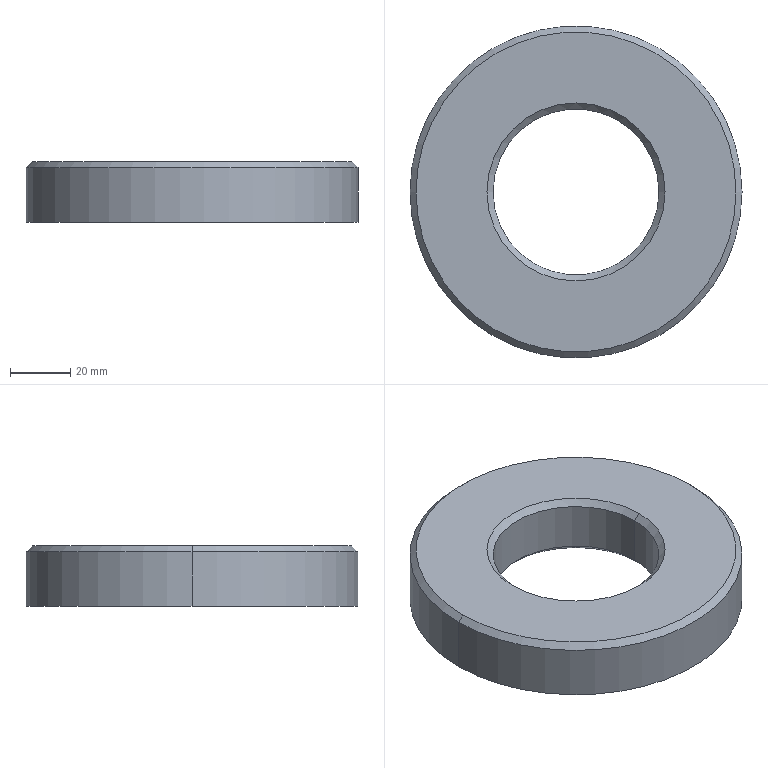Part | SolidWorks | features Chamfer 1, Extrusion 1 | 1 solid | 12 faces | box 110 x 110 x 20 mm | volume 141159 mm3 | cone 6 | cylinder 4 | plane 2 | commonest cylinder face diameters 55 x2 110 x2
STEP:
#1=CARTESIAN_POINT('',(53.,0.,20.));
#2=VERTEX_POINT('',#1);
#3=CARTESIAN_POINT('',(-53.,0.,20.));
#4=VERTEX_POINT('',#3);
#5=CARTESIAN_POINT('',(0.,0.,20.));
#6=DIRECTION('',(0.,0.,1.));
#7=DIRECTION('',(1.,0.,0.));
#8=AXIS2_PLACEMENT_3D('',#5,#6,#7);
#9=CIRCLE('',#8,53.);
#10=EDGE_CURVE('',#2,#4,#9,.T.);
#11=ORIENTED_EDGE('',*,*,#10,.F.);
#12=CARTESIAN_POINT('',(55.,0.,18.));
#13=VERTEX_POINT('',#12);
#14=CARTESIAN_POINT('',(53.,0.,20.));
#15=DIRECTION('',(0.7071,0.,-0.7071));
#16=VECTOR('',#15,1000.);
#17=LINE('',#14,#16);
#18=EDGE_CURVE('',#2,#13,#17,.T.);
#19=ORIENTED_EDGE('',*,*,#18,.T.);
#20=CARTESIAN_POINT('',(-55.,0.,18.));
#21=VERTEX_POINT('',#20);
#22=CARTESIAN_POINT('',(0.,0.,18.));
#23=DIRECTION('',(0.,0.,-1.));
#24=DIRECTION('',(1.,0.,0.));
#25=AXIS2_PLACEMENT_3D('',#22,#23,#24);
#26=CIRCLE('',#25,55.);
#27=EDGE_CURVE('',#21,#13,#26,.T.);
#28=ORIENTED_EDGE('',*,*,#27,.F.);
#29=CARTESIAN_POINT('',(-53.,0.,20.));
#30=DIRECTION('',(-0.7071,0.,-0.7071));
#31=VECTOR('',#30,1000.);
#32=LINE('',#29,#31);
#33=EDGE_CURVE('',#4,#21,#32,.T.);
#34=ORIENTED_EDGE('',*,*,#33,.F.);
#35=EDGE_LOOP('',(#11,#19,#28,#34));
#36=FACE_OUTER_BOUND('',#35,.T.);
#37=CARTESIAN_POINT('',(0.,0.,20.));
#38=DIRECTION('',(0.,0.,-1.));
#39=DIRECTION('',(-1.,0.,0.));
#40=AXIS2_PLACEMENT_3D('',#37,#38,#39);
#41=CONICAL_SURFACE('',#40,53.,0.7854);
#42=ADVANCED_FACE('',(#36),#41,.T.);
#43=CARTESIAN_POINT('',(-27.5,0.,18.));
#44=VERTEX_POINT('',#43);
#45=CARTESIAN_POINT('',(27.5,0.,18.));
#46=VERTEX_POINT('',#45);
#47=CARTESIAN_POINT('',(0.,0.,18.));
#48=DIRECTION('',(0.,0.,1.));
#49=DIRECTION('',(1.,0.,0.));
#50=AXIS2_PLACEMENT_3D('',#47,#48,#49);
#51=CIRCLE('',#50,27.5);
#52=EDGE_CURVE('',#44,#46,#51,.T.);
#53=ORIENTED_EDGE('',*,*,#52,.F.);
#54=CARTESIAN_POINT('',(-29.5,0.,20.));
#55=VERTEX_POINT('',#54);
#56=CARTESIAN_POINT('',(-27.5,0.,18.));
#57=DIRECTION('',(-0.7071,0.,0.7071));
#58=VECTOR('',#57,1000.);
#59=LINE('',#56,#58);
#60=EDGE_CURVE('',#44,#55,#59,.T.);
#61=ORIENTED_EDGE('',*,*,#60,.T.);
#62=CARTESIAN_POINT('',(29.5,0.,20.));
#63=VERTEX_POINT('',#62);
#64=CARTESIAN_POINT('',(0.,0.,20.));
#65=DIRECTION('',(0.,0.,-1.));
#66=DIRECTION('',(1.,0.,0.));
#67=AXIS2_PLACEMENT_3D('',#64,#65,#66);
#68=CIRCLE('',#67,29.5);
#69=EDGE_CURVE('',#63,#55,#68,.T.);
#70=ORIENTED_EDGE('',*,*,#69,.F.);
#71=CARTESIAN_POINT('',(27.5,0.,18.));
#72=DIRECTION('',(0.7071,0.,0.7071));
#73=VECTOR('',#72,1000.);
#74=LINE('',#71,#73);
#75=EDGE_CURVE('',#46,#63,#74,.T.);
#76=ORIENTED_EDGE('',*,*,#75,.F.);
#77=EDGE_LOOP('',(#53,#61,#70,#76));
#78=FACE_OUTER_BOUND('',#77,.T.);
#79=CARTESIAN_POINT('',(0.,0.,18.));
#80=DIRECTION('',(0.,0.,1.));
#81=DIRECTION('',(1.,0.,0.));
#82=AXIS2_PLACEMENT_3D('',#79,#80,#81);
#83=CONICAL_SURFACE('',#82,27.5,0.7854);
#84=ADVANCED_FACE('',(#78),#83,.F.);
#85=CARTESIAN_POINT('',(27.5,0.,2.));
#86=VERTEX_POINT('',#85);
#87=CARTESIAN_POINT('',(-27.5,0.,2.));
#88=VERTEX_POINT('',#87);
#89=CARTESIAN_POINT('',(0.,0.,2.));
#90=DIRECTION('',(0.,0.,-1.));
#91=DIRECTION('',(1.,0.,0.));
#92=AXIS2_PLACEMENT_3D('',#89,#90,#91);
#93=CIRCLE('',#92,27.5);
#94=EDGE_CURVE('',#86,#88,#93,.T.);
#95=ORIENTED_EDGE('',*,*,#94,.F.);
#96=CARTESIAN_POINT('',(29.5,0.,0.));
#97=VERTEX_POINT('',#96);
#98=CARTESIAN_POINT('',(29.5,0.,0.));
#99=DIRECTION('',(0.7071,0.,-0.7071));
#100=VECTOR('',#99,1000.);
#101=LINE('',#98,#100);
#102=EDGE_CURVE('',#86,#97,#101,.T.);
#103=ORIENTED_EDGE('',*,*,#102,.T.);
#104=CARTESIAN_POINT('',(-29.5,0.,0.));
#105=VERTEX_POINT('',#104);
#106=CARTESIAN_POINT('',(0.,0.,0.));
#107=DIRECTION('',(0.,0.,1.));
#108=DIRECTION('',(1.,0.,0.));
#109=AXIS2_PLACEMENT_3D('',#106,#107,#108);
#110=CIRCLE('',#109,29.5);
#111=EDGE_CURVE('',#105,#97,#110,.T.);
#112=ORIENTED_EDGE('',*,*,#111,.F.);
#113=CARTESIAN_POINT('',(-29.5,0.,0.));
#114=DIRECTION('',(-0.7071,0.,-0.7071));
#115=VECTOR('',#114,1000.);
#116=LINE('',#113,#115);
#117=EDGE_CURVE('',#88,#105,#116,.T.);
#118=ORIENTED_EDGE('',*,*,#117,.F.);
#119=EDGE_LOOP('',(#95,#103,#112,#118));
#120=FACE_OUTER_BOUND('',#119,.T.);
#121=CARTESIAN_POINT('',(0.,0.,0.));
#122=DIRECTION('',(0.,0.,-1.));
#123=DIRECTION('',(-1.,0.,0.));
#124=AXIS2_PLACEMENT_3D('',#121,#122,#123);
#125=CONICAL_SURFACE('',#124,29.5,0.7854);
#126=ADVANCED_FACE('',(#120),#125,.F.);
#127=ORIENTED_EDGE('',*,*,#52,.T.);
#128=CARTESIAN_POINT('',(27.5,0.,20.));
#129=DIRECTION('',(0.,0.,-1.));
#130=VECTOR('',#129,1000.);
#131=LINE('',#128,#130);
#132=EDGE_CURVE('',#46,#86,#131,.T.);
#133=ORIENTED_EDGE('',*,*,#132,.T.);
#134=ORIENTED_EDGE('',*,*,#94,.T.);
#135=CARTESIAN_POINT('',(-27.5,0.,20.));
#136=DIRECTION('',(0.,0.,-1.));
#137=VECTOR('',#136,1000.);
#138=LINE('',#135,#137);
#139=EDGE_CURVE('',#44,#88,#138,.T.);
#140=ORIENTED_EDGE('',*,*,#139,.F.);
#141=EDGE_LOOP('',(#127,#133,#134,#140));
#142=FACE_OUTER_BOUND('',#141,.T.);
#143=CARTESIAN_POINT('',(0.,0.,20.));
#144=DIRECTION('',(0.,0.,-1.));
#145=DIRECTION('',(-1.,0.,0.));
#146=AXIS2_PLACEMENT_3D('',#143,#144,#145);
#147=CYLINDRICAL_SURFACE('',#146,27.5);
#148=ADVANCED_FACE('',(#142),#147,.F.);
#149=ORIENTED_EDGE('',*,*,#27,.T.);
#150=CARTESIAN_POINT('',(55.,0.,0.));
#151=VERTEX_POINT('',#150);
#152=CARTESIAN_POINT('',(55.,0.,20.));
#153=DIRECTION('',(0.,0.,-1.));
#154=VECTOR('',#153,1000.);
#155=LINE('',#152,#154);
#156=EDGE_CURVE('',#13,#151,#155,.T.);
#157=ORIENTED_EDGE('',*,*,#156,.T.);
#158=CARTESIAN_POINT('',(-55.,0.,0.));
#159=VERTEX_POINT('',#158);
#160=CARTESIAN_POINT('',(0.,0.,0.));
#161=DIRECTION('',(0.,0.,1.));
#162=DIRECTION('',(1.,0.,0.));
#163=AXIS2_PLACEMENT_3D('',#160,#161,#162);
#164=CIRCLE('',#163,55.);
#165=EDGE_CURVE('',#151,#159,#164,.T.);
#166=ORIENTED_EDGE('',*,*,#165,.T.);
#167=CARTESIAN_POINT('',(-55.,0.,20.));
#168=DIRECTION('',(0.,0.,-1.));
#169=VECTOR('',#168,1000.);
#170=LINE('',#167,#169);
#171=EDGE_CURVE('',#21,#159,#170,.T.);
#172=ORIENTED_EDGE('',*,*,#171,.F.);
#173=EDGE_LOOP('',(#149,#157,#166,#172));
#174=FACE_OUTER_BOUND('',#173,.T.);
#175=CARTESIAN_POINT('',(0.,0.,20.));
#176=DIRECTION('',(0.,0.,-1.));
#177=DIRECTION('',(-1.,0.,0.));
#178=AXIS2_PLACEMENT_3D('',#175,#176,#177);
#179=CYLINDRICAL_SURFACE('',#178,55.);
#180=ADVANCED_FACE('',(#174),#179,.T.);
#181=ORIENTED_EDGE('',*,*,#69,.T.);
#182=CARTESIAN_POINT('',(0.,0.,20.));
#183=DIRECTION('',(0.,0.,-1.));
#184=DIRECTION('',(1.,0.,0.));
#185=AXIS2_PLACEMENT_3D('',#182,#183,#184);
#186=CIRCLE('',#185,29.5);
#187=EDGE_CURVE('',#55,#63,#186,.T.);
#188=ORIENTED_EDGE('',*,*,#187,.T.);
#189=EDGE_LOOP('',(#181,#188));
#190=FACE_BOUND('',#189,.T.);
#191=CARTESIAN_POINT('',(0.,0.,20.));
#192=DIRECTION('',(0.,0.,1.));
#193=DIRECTION('',(1.,0.,0.));
#194=AXIS2_PLACEMENT_3D('',#191,#192,#193);
#195=CIRCLE('',#194,53.);
#196=EDGE_CURVE('',#4,#2,#195,.T.);
#197=ORIENTED_EDGE('',*,*,#196,.T.);
#198=ORIENTED_EDGE('',*,*,#10,.T.);
#199=EDGE_LOOP('',(#197,#198));
#200=FACE_OUTER_BOUND('',#199,.T.);
#201=CARTESIAN_POINT('',(0.,0.,20.));
#202=DIRECTION('',(0.,0.,1.));
#203=DIRECTION('',(1.,0.,0.));
#204=AXIS2_PLACEMENT_3D('',#201,#202,#203);
#205=PLANE('',#204);
#206=ADVANCED_FACE('',(#190,#200),#205,.T.);
#207=ORIENTED_EDGE('',*,*,#111,.T.);
#208=CARTESIAN_POINT('',(0.,0.,0.));
#209=DIRECTION('',(0.,0.,1.));
#210=DIRECTION('',(1.,0.,0.));
#211=AXIS2_PLACEMENT_3D('',#208,#209,#210);
#212=CIRCLE('',#211,29.5);
#213=EDGE_CURVE('',#97,#105,#212,.T.);
#214=ORIENTED_EDGE('',*,*,#213,.T.);
#215=EDGE_LOOP('',(#207,#214));
#216=FACE_BOUND('',#215,.T.);
#217=CARTESIAN_POINT('',(0.,0.,0.));
#218=DIRECTION('',(0.,0.,1.));
#219=DIRECTION('',(1.,0.,0.));
#220=AXIS2_PLACEMENT_3D('',#217,#218,#219);
#221=CIRCLE('',#220,55.);
#222=EDGE_CURVE('',#159,#151,#221,.T.);
#223=ORIENTED_EDGE('',*,*,#222,.F.);
#224=ORIENTED_EDGE('',*,*,#165,.F.);
#225=EDGE_LOOP('',(#223,#224));
#226=FACE_OUTER_BOUND('',#225,.T.);
#227=CARTESIAN_POINT('',(0.,0.,0.));
#228=DIRECTION('',(0.,0.,1.));
#229=DIRECTION('',(1.,0.,0.));
#230=AXIS2_PLACEMENT_3D('',#227,#228,#229);
#231=PLANE('',#230);
#232=ADVANCED_FACE('',(#216,#226),#231,.F.);
#233=ORIENTED_EDGE('',*,*,#156,.F.);
#234=CARTESIAN_POINT('',(0.,0.,18.));
#235=DIRECTION('',(0.,0.,-1.));
#236=DIRECTION('',(1.,0.,0.));
#237=AXIS2_PLACEMENT_3D('',#234,#235,#236);
#238=CIRCLE('',#237,55.);
#239=EDGE_CURVE('',#13,#21,#238,.T.);
#240=ORIENTED_EDGE('',*,*,#239,.T.);
#241=ORIENTED_EDGE('',*,*,#171,.T.);
#242=ORIENTED_EDGE('',*,*,#222,.T.);
#243=EDGE_LOOP('',(#233,#240,#241,#242));
#244=FACE_OUTER_BOUND('',#243,.T.);
#245=CARTESIAN_POINT('',(0.,0.,20.));
#246=DIRECTION('',(0.,0.,-1.));
#247=DIRECTION('',(-1.,0.,0.));
#248=AXIS2_PLACEMENT_3D('',#245,#246,#247);
#249=CYLINDRICAL_SURFACE('',#248,55.);
#250=ADVANCED_FACE('',(#244),#249,.T.);
#251=ORIENTED_EDGE('',*,*,#132,.F.);
#252=CARTESIAN_POINT('',(0.,0.,18.));
#253=DIRECTION('',(0.,0.,1.));
#254=DIRECTION('',(1.,0.,0.));
#255=AXIS2_PLACEMENT_3D('',#252,#253,#254);
#256=CIRCLE('',#255,27.5);
#257=EDGE_CURVE('',#46,#44,#256,.T.);
#258=ORIENTED_EDGE('',*,*,#257,.T.);
#259=ORIENTED_EDGE('',*,*,#139,.T.);
#260=CARTESIAN_POINT('',(0.,0.,2.));
#261=DIRECTION('',(0.,0.,-1.));
#262=DIRECTION('',(1.,0.,0.));
#263=AXIS2_PLACEMENT_3D('',#260,#261,#262);
#264=CIRCLE('',#263,27.5);
#265=EDGE_CURVE('',#88,#86,#264,.T.);
#266=ORIENTED_EDGE('',*,*,#265,.T.);
#267=EDGE_LOOP('',(#251,#258,#259,#266));
#268=FACE_OUTER_BOUND('',#267,.T.);
#269=CARTESIAN_POINT('',(0.,0.,20.));
#270=DIRECTION('',(0.,0.,-1.));
#271=DIRECTION('',(-1.,0.,0.));
#272=AXIS2_PLACEMENT_3D('',#269,#270,#271);
#273=CYLINDRICAL_SURFACE('',#272,27.5);
#274=ADVANCED_FACE('',(#268),#273,.F.);
#275=ORIENTED_EDGE('',*,*,#102,.F.);
#276=ORIENTED_EDGE('',*,*,#265,.F.);
#277=ORIENTED_EDGE('',*,*,#117,.T.);
#278=ORIENTED_EDGE('',*,*,#213,.F.);
#279=EDGE_LOOP('',(#275,#276,#277,#278));
#280=FACE_OUTER_BOUND('',#279,.T.);
#281=CARTESIAN_POINT('',(0.,0.,0.));
#282=DIRECTION('',(0.,0.,-1.));
#283=DIRECTION('',(-1.,0.,0.));
#284=AXIS2_PLACEMENT_3D('',#281,#282,#283);
#285=CONICAL_SURFACE('',#284,29.5,0.7854);
#286=ADVANCED_FACE('',(#280),#285,.F.);
#287=ORIENTED_EDGE('',*,*,#60,.F.);
#288=ORIENTED_EDGE('',*,*,#257,.F.);
#289=ORIENTED_EDGE('',*,*,#75,.T.);
#290=ORIENTED_EDGE('',*,*,#187,.F.);
#291=EDGE_LOOP('',(#287,#288,#289,#290));
#292=FACE_OUTER_BOUND('',#291,.T.);
#293=CARTESIAN_POINT('',(0.,0.,18.));
#294=DIRECTION('',(0.,0.,1.));
#295=DIRECTION('',(1.,0.,0.));
#296=AXIS2_PLACEMENT_3D('',#293,#294,#295);
#297=CONICAL_SURFACE('',#296,27.5,0.7854);
#298=ADVANCED_FACE('',(#292),#297,.F.);
#299=ORIENTED_EDGE('',*,*,#18,.F.);
#300=ORIENTED_EDGE('',*,*,#196,.F.);
#301=ORIENTED_EDGE('',*,*,#33,.T.);
#302=ORIENTED_EDGE('',*,*,#239,.F.);
#303=EDGE_LOOP('',(#299,#300,#301,#302));
#304=FACE_OUTER_BOUND('',#303,.T.);
#305=CARTESIAN_POINT('',(0.,0.,20.));
#306=DIRECTION('',(0.,0.,-1.));
#307=DIRECTION('',(-1.,0.,0.));
#308=AXIS2_PLACEMENT_3D('',#305,#306,#307);
#309=CONICAL_SURFACE('',#308,53.,0.7854);
#310=ADVANCED_FACE('',(#304),#309,.T.);
#311=CLOSED_SHELL('',(#42,#84,#126,#148,#180,#206,#232,#250,#274,#286,#298,#310));
#312=MANIFOLD_SOLID_BREP('',#311);
#313=CARTESIAN_POINT('',(0.,0.,0.));
#314=DIRECTION('',(0.,0.,1.));
#315=DIRECTION('',(1.,0.,0.));
#316=AXIS2_PLACEMENT_3D('',#313,#314,#315);
#317=(LENGTH_UNIT()NAMED_UNIT(*)SI_UNIT(.MILLI.,.METRE.));
#318=UNCERTAINTY_MEASURE_WITH_UNIT(LENGTH_MEASURE(0.00001),#317,'','');
#319=(NAMED_UNIT(*)PLANE_ANGLE_UNIT()SI_UNIT($,.RADIAN.));
#320=(NAMED_UNIT(*)SI_UNIT($,.STERADIAN.)SOLID_ANGLE_UNIT());
#321=(GEOMETRIC_REPRESENTATION_CONTEXT(3)GLOBAL_UNCERTAINTY_ASSIGNED_CONTEXT((#318))GLOBAL_UNIT_ASSIGNED_CONTEXT((#317,#319,#320))REPRESENTATION_CONTEXT('',''));
#322=ADVANCED_BREP_SHAPE_REPRESENTATION('',(#312,#316),#321);